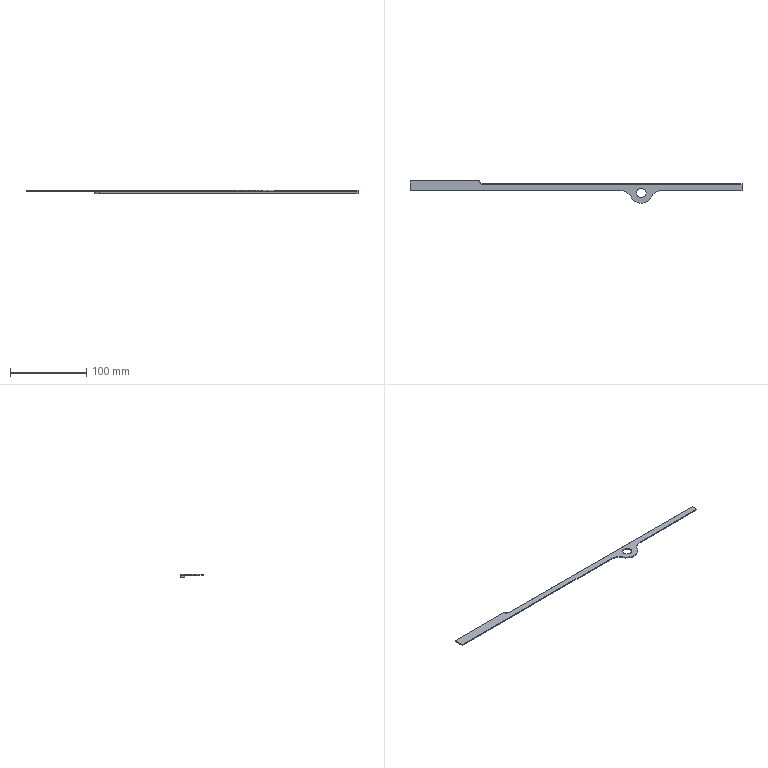Part | STEP file | gslz 2016.10.28-13_id958_x_t | 1 solid | 21 faces | box 436.271 x 29.5 x 4 mm | volume 6895 mm3 | plane 11 | cylinder 9 | torus 1 | commonest cylinder face diameters 30 x3 4 x2 2 x1 10 x1 12.3 x1 12.5 x1